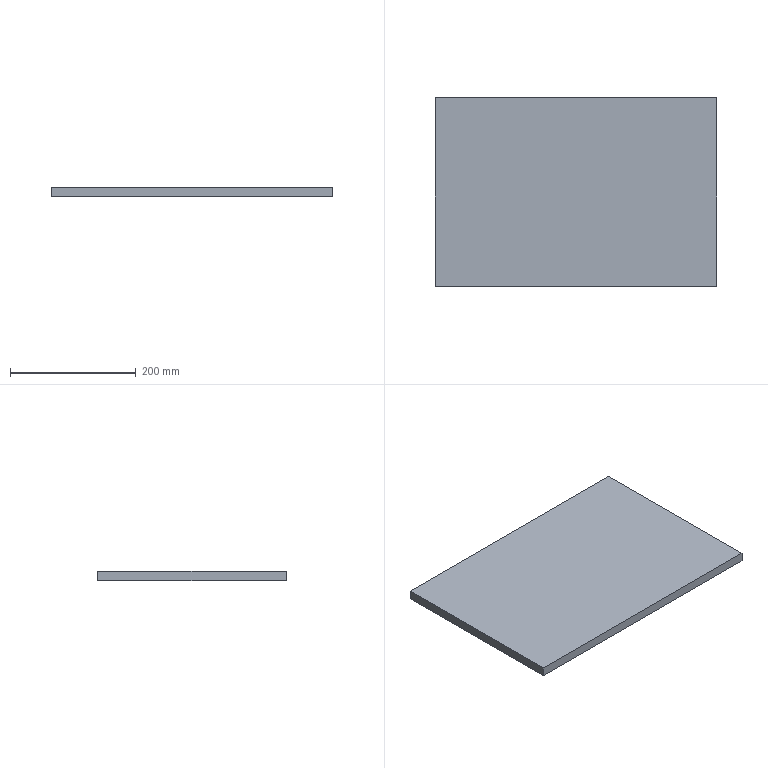Part | STEP file | Platform 1 base plate | 1 solid | 6 faces | box 448 x 300 x 15 mm | volume 2016000 mm3 | plane 6
STEP:
#1=CARTESIAN_POINT('',(224.,-150.,0.));
#2=VERTEX_POINT('',#1);
#3=CARTESIAN_POINT('',(224.,150.,0.));
#4=VERTEX_POINT('',#3);
#5=CARTESIAN_POINT('',(224.,150.,0.));
#6=DIRECTION('',(0.,1.,0.));
#7=VECTOR('',#6,1000.);
#8=LINE('',#5,#7);
#9=EDGE_CURVE('',#2,#4,#8,.T.);
#10=ORIENTED_EDGE('',*,*,#9,.T.);
#11=CARTESIAN_POINT('',(224.,150.,15.));
#12=VERTEX_POINT('',#11);
#13=CARTESIAN_POINT('',(224.,150.,15.));
#14=DIRECTION('',(0.,0.,-1.));
#15=VECTOR('',#14,1000.);
#16=LINE('',#13,#15);
#17=EDGE_CURVE('',#12,#4,#16,.T.);
#18=ORIENTED_EDGE('',*,*,#17,.F.);
#19=CARTESIAN_POINT('',(224.,-150.,15.));
#20=VERTEX_POINT('',#19);
#21=CARTESIAN_POINT('',(224.,150.,15.));
#22=DIRECTION('',(0.,1.,0.));
#23=VECTOR('',#22,1000.);
#24=LINE('',#21,#23);
#25=EDGE_CURVE('',#20,#12,#24,.T.);
#26=ORIENTED_EDGE('',*,*,#25,.F.);
#27=CARTESIAN_POINT('',(224.,-150.,15.));
#28=DIRECTION('',(0.,0.,-1.));
#29=VECTOR('',#28,1000.);
#30=LINE('',#27,#29);
#31=EDGE_CURVE('',#20,#2,#30,.T.);
#32=ORIENTED_EDGE('',*,*,#31,.T.);
#33=EDGE_LOOP('',(#10,#18,#26,#32));
#34=FACE_OUTER_BOUND('',#33,.T.);
#35=CARTESIAN_POINT('',(224.,150.,15.));
#36=DIRECTION('',(-1.,0.,0.));
#37=DIRECTION('',(0.,-1.,0.));
#38=AXIS2_PLACEMENT_3D('',#35,#36,#37);
#39=PLANE('',#38);
#40=ADVANCED_FACE('',(#34),#39,.F.);
#41=CARTESIAN_POINT('',(-224.,150.,0.));
#42=VERTEX_POINT('',#41);
#43=CARTESIAN_POINT('',(-224.,150.,0.));
#44=DIRECTION('',(-1.,0.,0.));
#45=VECTOR('',#44,1000.);
#46=LINE('',#43,#45);
#47=EDGE_CURVE('',#4,#42,#46,.T.);
#48=ORIENTED_EDGE('',*,*,#47,.T.);
#49=CARTESIAN_POINT('',(-224.,150.,15.));
#50=VERTEX_POINT('',#49);
#51=CARTESIAN_POINT('',(-224.,150.,15.));
#52=DIRECTION('',(0.,0.,-1.));
#53=VECTOR('',#52,1000.);
#54=LINE('',#51,#53);
#55=EDGE_CURVE('',#50,#42,#54,.T.);
#56=ORIENTED_EDGE('',*,*,#55,.F.);
#57=CARTESIAN_POINT('',(-224.,150.,15.));
#58=DIRECTION('',(-1.,0.,0.));
#59=VECTOR('',#58,1000.);
#60=LINE('',#57,#59);
#61=EDGE_CURVE('',#12,#50,#60,.T.);
#62=ORIENTED_EDGE('',*,*,#61,.F.);
#63=ORIENTED_EDGE('',*,*,#17,.T.);
#64=EDGE_LOOP('',(#48,#56,#62,#63));
#65=FACE_OUTER_BOUND('',#64,.T.);
#66=CARTESIAN_POINT('',(-224.,150.,15.));
#67=DIRECTION('',(0.,-1.,0.));
#68=DIRECTION('',(0.,0.,-1.));
#69=AXIS2_PLACEMENT_3D('',#66,#67,#68);
#70=PLANE('',#69);
#71=ADVANCED_FACE('',(#65),#70,.F.);
#72=CARTESIAN_POINT('',(-224.,-150.,0.));
#73=VERTEX_POINT('',#72);
#74=CARTESIAN_POINT('',(-224.,150.,0.));
#75=DIRECTION('',(0.,-1.,0.));
#76=VECTOR('',#75,1000.);
#77=LINE('',#74,#76);
#78=EDGE_CURVE('',#42,#73,#77,.T.);
#79=ORIENTED_EDGE('',*,*,#78,.T.);
#80=CARTESIAN_POINT('',(-224.,-150.,15.));
#81=VERTEX_POINT('',#80);
#82=CARTESIAN_POINT('',(-224.,-150.,15.));
#83=DIRECTION('',(0.,0.,-1.));
#84=VECTOR('',#83,1000.);
#85=LINE('',#82,#84);
#86=EDGE_CURVE('',#81,#73,#85,.T.);
#87=ORIENTED_EDGE('',*,*,#86,.F.);
#88=CARTESIAN_POINT('',(-224.,150.,15.));
#89=DIRECTION('',(0.,-1.,0.));
#90=VECTOR('',#89,1000.);
#91=LINE('',#88,#90);
#92=EDGE_CURVE('',#50,#81,#91,.T.);
#93=ORIENTED_EDGE('',*,*,#92,.F.);
#94=ORIENTED_EDGE('',*,*,#55,.T.);
#95=EDGE_LOOP('',(#79,#87,#93,#94));
#96=FACE_OUTER_BOUND('',#95,.T.);
#97=CARTESIAN_POINT('',(-224.,150.,15.));
#98=DIRECTION('',(1.,0.,0.));
#99=DIRECTION('',(0.,1.,0.));
#100=AXIS2_PLACEMENT_3D('',#97,#98,#99);
#101=PLANE('',#100);
#102=ADVANCED_FACE('',(#96),#101,.F.);
#103=CARTESIAN_POINT('',(-224.,-150.,0.));
#104=DIRECTION('',(1.,0.,0.));
#105=VECTOR('',#104,1000.);
#106=LINE('',#103,#105);
#107=EDGE_CURVE('',#73,#2,#106,.T.);
#108=ORIENTED_EDGE('',*,*,#107,.T.);
#109=ORIENTED_EDGE('',*,*,#31,.F.);
#110=CARTESIAN_POINT('',(-224.,-150.,15.));
#111=DIRECTION('',(1.,0.,0.));
#112=VECTOR('',#111,1000.);
#113=LINE('',#110,#112);
#114=EDGE_CURVE('',#81,#20,#113,.T.);
#115=ORIENTED_EDGE('',*,*,#114,.F.);
#116=ORIENTED_EDGE('',*,*,#86,.T.);
#117=EDGE_LOOP('',(#108,#109,#115,#116));
#118=FACE_OUTER_BOUND('',#117,.T.);
#119=CARTESIAN_POINT('',(-224.,-150.,15.));
#120=DIRECTION('',(0.,1.,0.));
#121=DIRECTION('',(0.,0.,1.));
#122=AXIS2_PLACEMENT_3D('',#119,#120,#121);
#123=PLANE('',#122);
#124=ADVANCED_FACE('',(#118),#123,.F.);
#125=ORIENTED_EDGE('',*,*,#25,.T.);
#126=ORIENTED_EDGE('',*,*,#61,.T.);
#127=ORIENTED_EDGE('',*,*,#92,.T.);
#128=ORIENTED_EDGE('',*,*,#114,.T.);
#129=EDGE_LOOP('',(#125,#126,#127,#128));
#130=FACE_OUTER_BOUND('',#129,.T.);
#131=CARTESIAN_POINT('',(0.,0.,15.));
#132=DIRECTION('',(0.,0.,1.));
#133=DIRECTION('',(1.,0.,0.));
#134=AXIS2_PLACEMENT_3D('',#131,#132,#133);
#135=PLANE('',#134);
#136=ADVANCED_FACE('',(#130),#135,.T.);
#137=ORIENTED_EDGE('',*,*,#9,.F.);
#138=ORIENTED_EDGE('',*,*,#107,.F.);
#139=ORIENTED_EDGE('',*,*,#78,.F.);
#140=ORIENTED_EDGE('',*,*,#47,.F.);
#141=EDGE_LOOP('',(#137,#138,#139,#140));
#142=FACE_OUTER_BOUND('',#141,.T.);
#143=CARTESIAN_POINT('',(0.,0.,0.));
#144=DIRECTION('',(0.,0.,1.));
#145=DIRECTION('',(1.,0.,0.));
#146=AXIS2_PLACEMENT_3D('',#143,#144,#145);
#147=PLANE('',#146);
#148=ADVANCED_FACE('',(#142),#147,.F.);
#149=CLOSED_SHELL('',(#40,#71,#102,#124,#136,#148));
#150=MANIFOLD_SOLID_BREP('',#149);
#151=CARTESIAN_POINT('',(0.,0.,0.));
#152=DIRECTION('',(0.,0.,1.));
#153=DIRECTION('',(1.,0.,0.));
#154=AXIS2_PLACEMENT_3D('',#151,#152,#153);
#155=(LENGTH_UNIT()NAMED_UNIT(*)SI_UNIT(.MILLI.,.METRE.));
#156=UNCERTAINTY_MEASURE_WITH_UNIT(LENGTH_MEASURE(0.00001),#155,'','');
#157=(NAMED_UNIT(*)PLANE_ANGLE_UNIT()SI_UNIT($,.RADIAN.));
#158=(NAMED_UNIT(*)SI_UNIT($,.STERADIAN.)SOLID_ANGLE_UNIT());
#159=(GEOMETRIC_REPRESENTATION_CONTEXT(3)GLOBAL_UNCERTAINTY_ASSIGNED_CONTEXT((#156))GLOBAL_UNIT_ASSIGNED_CONTEXT((#155,#157,#158))REPRESENTATION_CONTEXT('',''));
#160=ADVANCED_BREP_SHAPE_REPRESENTATION('',(#150,#154),#159);